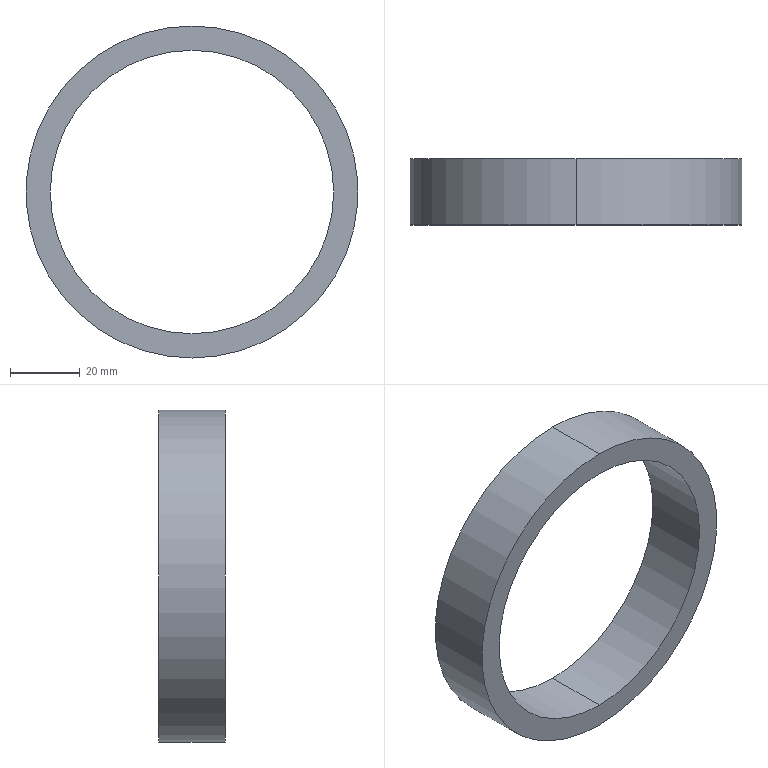Part | STEP file | 1 solid | 6 faces | box 95.525 x 19 x 95.525 mm | volume 36998 mm3 | cylinder 4 | plane 2 | commonest cylinder face diameters 81.521 x2 95.525 x2
STEP:
#1=CARTESIAN_POINT('',(0.,0.,0.));
#2=DIRECTION('',(0.,0.,1.));
#3=DIRECTION('',(1.,0.,0.));
#4=AXIS2_PLACEMENT_3D('',#1,#2,#3);
#5=CARTESIAN_POINT('',(340.649,373.014,205.345));
#6=VERTEX_POINT('',#5);
#7=CARTESIAN_POINT('',(340.649,354.014,205.345));
#8=VERTEX_POINT('',#7);
#9=CARTESIAN_POINT('',(340.649,373.014,205.345));
#10=DIRECTION('',(0.,-1.,0.));
#11=VECTOR('',#10,1.);
#12=LINE('',#9,#11);
#13=CARTESIAN_POINT('',(340.649,373.014,246.106));
#14=DIRECTION('',(0.,-1.,0.));
#15=DIRECTION('',(0.,0.,-1.));
#16=AXIS2_PLACEMENT_3D('',#13,#14,#15);
#17=CYLINDRICAL_SURFACE('',#16,40.761);
#18=CARTESIAN_POINT('',(6.283,0.));
#19=DIRECTION('',(0.,1.));
#20=VECTOR('',#19,1.);
#21=LINE('',#18,#20);
#22=(GEOMETRIC_REPRESENTATION_CONTEXT(2)PARAMETRIC_REPRESENTATION_CONTEXT()REPRESENTATION_CONTEXT('',''));
#23=DEFINITIONAL_REPRESENTATION('',(#21),#22);
#24=PCURVE('',#17,#23);
#25=CARTESIAN_POINT('',(340.649,373.014,246.106));
#26=DIRECTION('',(0.,-1.,0.));
#27=DIRECTION('',(0.,0.,-1.));
#28=AXIS2_PLACEMENT_3D('',#25,#26,#27);
#29=CYLINDRICAL_SURFACE('',#28,40.761);
#30=CARTESIAN_POINT('',(0.,0.));
#31=DIRECTION('',(0.,1.));
#32=VECTOR('',#31,1.);
#33=LINE('',#30,#32);
#34=(GEOMETRIC_REPRESENTATION_CONTEXT(2)PARAMETRIC_REPRESENTATION_CONTEXT()REPRESENTATION_CONTEXT('',''));
#35=DEFINITIONAL_REPRESENTATION('',(#33),#34);
#36=PCURVE('',#29,#35);
#37=SURFACE_CURVE('',#12,(#24,#36),.PCURVE_S1.);
#38=EDGE_CURVE('',#6,#8,#37,.T.);
#39=ORIENTED_EDGE('',*,*,#38,.T.);
#40=CARTESIAN_POINT('',(340.649,354.014,286.866));
#41=VERTEX_POINT('',#40);
#42=CARTESIAN_POINT('',(340.649,354.014,246.106));
#43=DIRECTION('',(0.,1.,0.));
#44=DIRECTION('',(0.,0.,1.));
#45=AXIS2_PLACEMENT_3D('',#42,#43,#44);
#46=CIRCLE('',#45,40.761);
#47=CARTESIAN_POINT('',(9.425,19.));
#48=DIRECTION('',(-1.,0.));
#49=VECTOR('',#48,1.);
#50=LINE('',#47,#49);
#51=(GEOMETRIC_REPRESENTATION_CONTEXT(2)PARAMETRIC_REPRESENTATION_CONTEXT()REPRESENTATION_CONTEXT('',''));
#52=DEFINITIONAL_REPRESENTATION('',(#50),#51);
#53=PCURVE('',#17,#52);
#54=CARTESIAN_POINT('',(340.649,354.014,246.106));
#55=DIRECTION('',(0.,1.,0.));
#56=DIRECTION('',(0.,0.,1.));
#57=AXIS2_PLACEMENT_3D('',#54,#55,#56);
#58=PLANE('',#57);
#59=CARTESIAN_POINT('',(0.,0.));
#60=DIRECTION('',(1.,0.));
#61=AXIS2_PLACEMENT_2D('',#59,#60);
#62=CIRCLE('',#61,40.761);
#63=(GEOMETRIC_REPRESENTATION_CONTEXT(2)PARAMETRIC_REPRESENTATION_CONTEXT()REPRESENTATION_CONTEXT('',''));
#64=DEFINITIONAL_REPRESENTATION('',(#62),#63);
#65=PCURVE('',#58,#64);
#66=SURFACE_CURVE('',#46,(#53,#65),.PCURVE_S1.);
#67=EDGE_CURVE('',#8,#41,#66,.T.);
#68=ORIENTED_EDGE('',*,*,#67,.T.);
#69=CARTESIAN_POINT('',(340.649,373.014,286.866));
#70=VERTEX_POINT('',#69);
#71=CARTESIAN_POINT('',(340.649,373.014,286.866));
#72=DIRECTION('',(0.,-1.,0.));
#73=VECTOR('',#72,1.);
#74=LINE('',#71,#73);
#75=CARTESIAN_POINT('',(3.142,0.));
#76=DIRECTION('',(0.,1.));
#77=VECTOR('',#76,1.);
#78=LINE('',#75,#77);
#79=(GEOMETRIC_REPRESENTATION_CONTEXT(2)PARAMETRIC_REPRESENTATION_CONTEXT()REPRESENTATION_CONTEXT('',''));
#80=DEFINITIONAL_REPRESENTATION('',(#78),#79);
#81=PCURVE('',#17,#80);
#82=CARTESIAN_POINT('',(3.142,0.));
#83=DIRECTION('',(0.,1.));
#84=VECTOR('',#83,1.);
#85=LINE('',#82,#84);
#86=(GEOMETRIC_REPRESENTATION_CONTEXT(2)PARAMETRIC_REPRESENTATION_CONTEXT()REPRESENTATION_CONTEXT('',''));
#87=DEFINITIONAL_REPRESENTATION('',(#85),#86);
#88=PCURVE('',#29,#87);
#89=SURFACE_CURVE('',#74,(#81,#88),.PCURVE_S1.);
#90=EDGE_CURVE('',#70,#41,#89,.T.);
#91=ORIENTED_EDGE('',*,*,#90,.F.);
#92=CARTESIAN_POINT('',(340.649,373.014,246.106));
#93=DIRECTION('',(0.,1.,0.));
#94=DIRECTION('',(0.,0.,1.));
#95=AXIS2_PLACEMENT_3D('',#92,#93,#94);
#96=CIRCLE('',#95,40.761);
#97=CARTESIAN_POINT('',(9.425,0.));
#98=DIRECTION('',(-1.,0.));
#99=VECTOR('',#98,1.);
#100=LINE('',#97,#99);
#101=(GEOMETRIC_REPRESENTATION_CONTEXT(2)PARAMETRIC_REPRESENTATION_CONTEXT()REPRESENTATION_CONTEXT('',''));
#102=DEFINITIONAL_REPRESENTATION('',(#100),#101);
#103=PCURVE('',#17,#102);
#104=CARTESIAN_POINT('',(340.649,373.014,246.106));
#105=DIRECTION('',(0.,1.,0.));
#106=DIRECTION('',(0.,0.,1.));
#107=AXIS2_PLACEMENT_3D('',#104,#105,#106);
#108=PLANE('',#107);
#109=CARTESIAN_POINT('',(0.,0.));
#110=DIRECTION('',(1.,0.));
#111=AXIS2_PLACEMENT_2D('',#109,#110);
#112=CIRCLE('',#111,40.761);
#113=(GEOMETRIC_REPRESENTATION_CONTEXT(2)PARAMETRIC_REPRESENTATION_CONTEXT()REPRESENTATION_CONTEXT('',''));
#114=DEFINITIONAL_REPRESENTATION('',(#112),#113);
#115=PCURVE('',#108,#114);
#116=SURFACE_CURVE('',#96,(#103,#115),.PCURVE_S1.);
#117=EDGE_CURVE('',#6,#70,#116,.T.);
#118=ORIENTED_EDGE('',*,*,#117,.F.);
#119=EDGE_LOOP('',(#39,#68,#91,#118));
#120=FACE_BOUND('',#119,.F.);
#121=ADVANCED_FACE('',(#120),#17,.F.);
#122=CARTESIAN_POINT('',(340.649,373.014,293.868));
#123=VERTEX_POINT('',#122);
#124=CARTESIAN_POINT('',(340.649,373.014,198.343));
#125=VERTEX_POINT('',#124);
#126=CARTESIAN_POINT('',(340.649,373.014,246.106));
#127=DIRECTION('',(0.,1.,0.));
#128=DIRECTION('',(0.,0.,1.));
#129=AXIS2_PLACEMENT_3D('',#126,#127,#128);
#130=CIRCLE('',#129,47.762);
#131=CARTESIAN_POINT('',(340.649,373.014,246.106));
#132=DIRECTION('',(0.,-1.,0.));
#133=DIRECTION('',(0.,0.,-1.));
#134=AXIS2_PLACEMENT_3D('',#131,#132,#133);
#135=CYLINDRICAL_SURFACE('',#134,47.762);
#136=CARTESIAN_POINT('',(3.142,0.));
#137=DIRECTION('',(-1.,0.));
#138=VECTOR('',#137,1.);
#139=LINE('',#136,#138);
#140=(GEOMETRIC_REPRESENTATION_CONTEXT(2)PARAMETRIC_REPRESENTATION_CONTEXT()REPRESENTATION_CONTEXT('',''));
#141=DEFINITIONAL_REPRESENTATION('',(#139),#140);
#142=PCURVE('',#135,#141);
#143=CARTESIAN_POINT('',(0.,0.));
#144=DIRECTION('',(1.,0.));
#145=AXIS2_PLACEMENT_2D('',#143,#144);
#146=CIRCLE('',#145,47.762);
#147=(GEOMETRIC_REPRESENTATION_CONTEXT(2)PARAMETRIC_REPRESENTATION_CONTEXT()REPRESENTATION_CONTEXT('',''));
#148=DEFINITIONAL_REPRESENTATION('',(#146),#147);
#149=PCURVE('',#108,#148);
#150=SURFACE_CURVE('',#130,(#142,#149),.PCURVE_S1.);
#151=EDGE_CURVE('',#123,#125,#150,.T.);
#152=ORIENTED_EDGE('',*,*,#151,.F.);
#153=CARTESIAN_POINT('',(340.649,354.014,293.868));
#154=VERTEX_POINT('',#153);
#155=CARTESIAN_POINT('',(340.649,373.014,293.868));
#156=DIRECTION('',(0.,-1.,0.));
#157=VECTOR('',#156,1.);
#158=LINE('',#155,#157);
#159=CARTESIAN_POINT('',(3.142,0.));
#160=DIRECTION('',(0.,1.));
#161=VECTOR('',#160,1.);
#162=LINE('',#159,#161);
#163=(GEOMETRIC_REPRESENTATION_CONTEXT(2)PARAMETRIC_REPRESENTATION_CONTEXT()REPRESENTATION_CONTEXT('',''));
#164=DEFINITIONAL_REPRESENTATION('',(#162),#163);
#165=PCURVE('',#135,#164);
#166=CARTESIAN_POINT('',(340.649,373.014,246.106));
#167=DIRECTION('',(0.,-1.,0.));
#168=DIRECTION('',(0.,0.,-1.));
#169=AXIS2_PLACEMENT_3D('',#166,#167,#168);
#170=CYLINDRICAL_SURFACE('',#169,47.762);
#171=CARTESIAN_POINT('',(3.142,0.));
#172=DIRECTION('',(0.,1.));
#173=VECTOR('',#172,1.);
#174=LINE('',#171,#173);
#175=(GEOMETRIC_REPRESENTATION_CONTEXT(2)PARAMETRIC_REPRESENTATION_CONTEXT()REPRESENTATION_CONTEXT('',''));
#176=DEFINITIONAL_REPRESENTATION('',(#174),#175);
#177=PCURVE('',#170,#176);
#178=SURFACE_CURVE('',#158,(#165,#177),.PCURVE_S1.);
#179=EDGE_CURVE('',#123,#154,#178,.T.);
#180=ORIENTED_EDGE('',*,*,#179,.T.);
#181=CARTESIAN_POINT('',(340.649,354.014,198.343));
#182=VERTEX_POINT('',#181);
#183=CARTESIAN_POINT('',(340.649,354.014,246.106));
#184=DIRECTION('',(0.,1.,0.));
#185=DIRECTION('',(0.,0.,1.));
#186=AXIS2_PLACEMENT_3D('',#183,#184,#185);
#187=CIRCLE('',#186,47.762);
#188=CARTESIAN_POINT('',(3.142,19.));
#189=DIRECTION('',(-1.,0.));
#190=VECTOR('',#189,1.);
#191=LINE('',#188,#190);
#192=(GEOMETRIC_REPRESENTATION_CONTEXT(2)PARAMETRIC_REPRESENTATION_CONTEXT()REPRESENTATION_CONTEXT('',''));
#193=DEFINITIONAL_REPRESENTATION('',(#191),#192);
#194=PCURVE('',#135,#193);
#195=CARTESIAN_POINT('',(0.,0.));
#196=DIRECTION('',(1.,0.));
#197=AXIS2_PLACEMENT_2D('',#195,#196);
#198=CIRCLE('',#197,47.762);
#199=(GEOMETRIC_REPRESENTATION_CONTEXT(2)PARAMETRIC_REPRESENTATION_CONTEXT()REPRESENTATION_CONTEXT('',''));
#200=DEFINITIONAL_REPRESENTATION('',(#198),#199);
#201=PCURVE('',#58,#200);
#202=SURFACE_CURVE('',#187,(#194,#201),.PCURVE_S1.);
#203=EDGE_CURVE('',#154,#182,#202,.T.);
#204=ORIENTED_EDGE('',*,*,#203,.T.);
#205=CARTESIAN_POINT('',(340.649,373.014,198.343));
#206=DIRECTION('',(0.,-1.,0.));
#207=VECTOR('',#206,1.);
#208=LINE('',#205,#207);
#209=CARTESIAN_POINT('',(0.,0.));
#210=DIRECTION('',(0.,1.));
#211=VECTOR('',#210,1.);
#212=LINE('',#209,#211);
#213=(GEOMETRIC_REPRESENTATION_CONTEXT(2)PARAMETRIC_REPRESENTATION_CONTEXT()REPRESENTATION_CONTEXT('',''));
#214=DEFINITIONAL_REPRESENTATION('',(#212),#213);
#215=PCURVE('',#135,#214);
#216=CARTESIAN_POINT('',(6.283,0.));
#217=DIRECTION('',(0.,1.));
#218=VECTOR('',#217,1.);
#219=LINE('',#216,#218);
#220=(GEOMETRIC_REPRESENTATION_CONTEXT(2)PARAMETRIC_REPRESENTATION_CONTEXT()REPRESENTATION_CONTEXT('',''));
#221=DEFINITIONAL_REPRESENTATION('',(#219),#220);
#222=PCURVE('',#170,#221);
#223=SURFACE_CURVE('',#208,(#215,#222),.PCURVE_S1.);
#224=EDGE_CURVE('',#125,#182,#223,.T.);
#225=ORIENTED_EDGE('',*,*,#224,.F.);
#226=EDGE_LOOP('',(#152,#180,#204,#225));
#227=FACE_BOUND('',#226,.T.);
#228=ADVANCED_FACE('',(#227),#135,.T.);
#229=CARTESIAN_POINT('',(340.649,373.014,246.106));
#230=DIRECTION('',(0.,1.,0.));
#231=DIRECTION('',(0.,0.,1.));
#232=AXIS2_PLACEMENT_3D('',#229,#230,#231);
#233=CIRCLE('',#232,47.762);
#234=CARTESIAN_POINT('',(0.,0.));
#235=DIRECTION('',(1.,0.));
#236=AXIS2_PLACEMENT_2D('',#234,#235);
#237=CIRCLE('',#236,47.762);
#238=(GEOMETRIC_REPRESENTATION_CONTEXT(2)PARAMETRIC_REPRESENTATION_CONTEXT()REPRESENTATION_CONTEXT('',''));
#239=DEFINITIONAL_REPRESENTATION('',(#237),#238);
#240=PCURVE('',#108,#239);
#241=CARTESIAN_POINT('',(9.425,0.));
#242=DIRECTION('',(-1.,0.));
#243=VECTOR('',#242,1.);
#244=LINE('',#241,#243);
#245=(GEOMETRIC_REPRESENTATION_CONTEXT(2)PARAMETRIC_REPRESENTATION_CONTEXT()REPRESENTATION_CONTEXT('',''));
#246=DEFINITIONAL_REPRESENTATION('',(#244),#245);
#247=PCURVE('',#170,#246);
#248=SURFACE_CURVE('',#233,(#240,#247),.PCURVE_S1.);
#249=EDGE_CURVE('',#125,#123,#248,.T.);
#250=ORIENTED_EDGE('',*,*,#249,.T.);
#251=ORIENTED_EDGE('',*,*,#151,.T.);
#252=EDGE_LOOP('',(#250,#251));
#253=FACE_BOUND('',#252,.T.);
#254=ORIENTED_EDGE('',*,*,#117,.F.);
#255=CARTESIAN_POINT('',(340.649,373.014,246.106));
#256=DIRECTION('',(0.,1.,0.));
#257=DIRECTION('',(0.,0.,1.));
#258=AXIS2_PLACEMENT_3D('',#255,#256,#257);
#259=CIRCLE('',#258,40.761);
#260=CARTESIAN_POINT('',(0.,0.));
#261=DIRECTION('',(1.,0.));
#262=AXIS2_PLACEMENT_2D('',#260,#261);
#263=CIRCLE('',#262,40.761);
#264=(GEOMETRIC_REPRESENTATION_CONTEXT(2)PARAMETRIC_REPRESENTATION_CONTEXT()REPRESENTATION_CONTEXT('',''));
#265=DEFINITIONAL_REPRESENTATION('',(#263),#264);
#266=PCURVE('',#108,#265);
#267=CARTESIAN_POINT('',(3.142,0.));
#268=DIRECTION('',(-1.,0.));
#269=VECTOR('',#268,1.);
#270=LINE('',#267,#269);
#271=(GEOMETRIC_REPRESENTATION_CONTEXT(2)PARAMETRIC_REPRESENTATION_CONTEXT()REPRESENTATION_CONTEXT('',''));
#272=DEFINITIONAL_REPRESENTATION('',(#270),#271);
#273=PCURVE('',#29,#272);
#274=SURFACE_CURVE('',#259,(#266,#273),.PCURVE_S1.);
#275=EDGE_CURVE('',#70,#6,#274,.T.);
#276=ORIENTED_EDGE('',*,*,#275,.F.);
#277=EDGE_LOOP('',(#254,#276));
#278=FACE_BOUND('',#277,.T.);
#279=ADVANCED_FACE('',(#253,#278),#108,.T.);
#280=CARTESIAN_POINT('',(340.649,354.014,246.106));
#281=DIRECTION('',(0.,1.,0.));
#282=DIRECTION('',(0.,0.,1.));
#283=AXIS2_PLACEMENT_3D('',#280,#281,#282);
#284=CIRCLE('',#283,47.762);
#285=CARTESIAN_POINT('',(0.,0.));
#286=DIRECTION('',(1.,0.));
#287=AXIS2_PLACEMENT_2D('',#285,#286);
#288=CIRCLE('',#287,47.762);
#289=(GEOMETRIC_REPRESENTATION_CONTEXT(2)PARAMETRIC_REPRESENTATION_CONTEXT()REPRESENTATION_CONTEXT('',''));
#290=DEFINITIONAL_REPRESENTATION('',(#288),#289);
#291=PCURVE('',#58,#290);
#292=CARTESIAN_POINT('',(9.425,19.));
#293=DIRECTION('',(-1.,0.));
#294=VECTOR('',#293,1.);
#295=LINE('',#292,#294);
#296=(GEOMETRIC_REPRESENTATION_CONTEXT(2)PARAMETRIC_REPRESENTATION_CONTEXT()REPRESENTATION_CONTEXT('',''));
#297=DEFINITIONAL_REPRESENTATION('',(#295),#296);
#298=PCURVE('',#170,#297);
#299=SURFACE_CURVE('',#284,(#291,#298),.PCURVE_S1.);
#300=EDGE_CURVE('',#182,#154,#299,.T.);
#301=ORIENTED_EDGE('',*,*,#300,.F.);
#302=ORIENTED_EDGE('',*,*,#203,.F.);
#303=EDGE_LOOP('',(#301,#302));
#304=FACE_BOUND('',#303,.T.);
#305=ORIENTED_EDGE('',*,*,#67,.T.);
#306=CARTESIAN_POINT('',(340.649,354.014,246.106));
#307=DIRECTION('',(0.,1.,0.));
#308=DIRECTION('',(0.,0.,1.));
#309=AXIS2_PLACEMENT_3D('',#306,#307,#308);
#310=CIRCLE('',#309,40.761);
#311=CARTESIAN_POINT('',(0.,0.));
#312=DIRECTION('',(1.,0.));
#313=AXIS2_PLACEMENT_2D('',#311,#312);
#314=CIRCLE('',#313,40.761);
#315=(GEOMETRIC_REPRESENTATION_CONTEXT(2)PARAMETRIC_REPRESENTATION_CONTEXT()REPRESENTATION_CONTEXT('',''));
#316=DEFINITIONAL_REPRESENTATION('',(#314),#315);
#317=PCURVE('',#58,#316);
#318=CARTESIAN_POINT('',(3.142,19.));
#319=DIRECTION('',(-1.,0.));
#320=VECTOR('',#319,1.);
#321=LINE('',#318,#320);
#322=(GEOMETRIC_REPRESENTATION_CONTEXT(2)PARAMETRIC_REPRESENTATION_CONTEXT()REPRESENTATION_CONTEXT('',''));
#323=DEFINITIONAL_REPRESENTATION('',(#321),#322);
#324=PCURVE('',#29,#323);
#325=SURFACE_CURVE('',#310,(#317,#324),.PCURVE_S1.);
#326=EDGE_CURVE('',#41,#8,#325,.T.);
#327=ORIENTED_EDGE('',*,*,#326,.T.);
#328=EDGE_LOOP('',(#305,#327));
#329=FACE_BOUND('',#328,.T.);
#330=ADVANCED_FACE('',(#304,#329),#58,.F.);
#331=ORIENTED_EDGE('',*,*,#179,.F.);
#332=ORIENTED_EDGE('',*,*,#249,.F.);
#333=ORIENTED_EDGE('',*,*,#224,.T.);
#334=ORIENTED_EDGE('',*,*,#300,.T.);
#335=EDGE_LOOP('',(#331,#332,#333,#334));
#336=FACE_BOUND('',#335,.T.);
#337=ADVANCED_FACE('',(#336),#170,.T.);
#338=ORIENTED_EDGE('',*,*,#326,.T.);
#339=ORIENTED_EDGE('',*,*,#38,.F.);
#340=ORIENTED_EDGE('',*,*,#275,.F.);
#341=ORIENTED_EDGE('',*,*,#90,.T.);
#342=EDGE_LOOP('',(#338,#339,#340,#341));
#343=FACE_BOUND('',#342,.F.);
#344=ADVANCED_FACE('',(#343),#29,.F.);
#345=CLOSED_SHELL('',(#121,#228,#279,#330,#337,#344));
#346=MANIFOLD_SOLID_BREP('',#345);
#347=(LENGTH_UNIT()NAMED_UNIT(*)SI_UNIT(.MILLI.,.METRE.));
#348=UNCERTAINTY_MEASURE_WITH_UNIT(LENGTH_MEASURE(0.0000001),#347,'','');
#349=(NAMED_UNIT(*)PLANE_ANGLE_UNIT()SI_UNIT($,.RADIAN.));
#350=(NAMED_UNIT(*)SI_UNIT($,.STERADIAN.)SOLID_ANGLE_UNIT());
#351=(GEOMETRIC_REPRESENTATION_CONTEXT(3)GLOBAL_UNCERTAINTY_ASSIGNED_CONTEXT((#348))GLOBAL_UNIT_ASSIGNED_CONTEXT((#347,#349,#350))REPRESENTATION_CONTEXT('',''));
#352=ADVANCED_BREP_SHAPE_REPRESENTATION('',(#4,#346),#351);